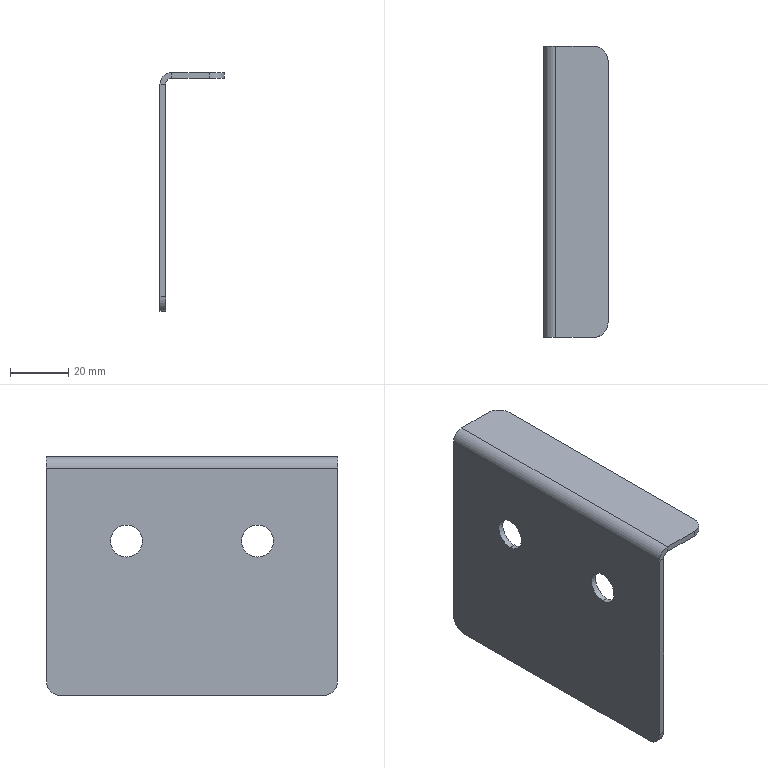Part | SolidWorks | features Fillet 1, FlatPattern 1, ICE 1, SMBaseFlange 1, SheetMetal 1 | 1 solid | 22 faces | box 22 x 100 x 82 mm | volume 19719 mm3 | plane 12 | cylinder 10 | commonest cylinder face diameters 10 x4 11 x4 4 x1 8 x1
STEP:
#1=CARTESIAN_POINT('',(0.,22.5,-32.5));
#2=VERTEX_POINT('',#1);
#3=CARTESIAN_POINT('',(0.,22.5,-21.5));
#4=VERTEX_POINT('',#3);
#5=CARTESIAN_POINT('',(0.,22.5,-27.));
#6=DIRECTION('',(-1.,0.,0.));
#7=DIRECTION('',(0.,0.,1.));
#8=AXIS2_PLACEMENT_3D('',#5,#6,#7);
#9=CIRCLE('',#8,5.5);
#10=EDGE_CURVE('',#2,#4,#9,.T.);
#11=ORIENTED_EDGE('',*,*,#10,.F.);
#12=CARTESIAN_POINT('',(-2.,22.5,-32.5));
#13=VERTEX_POINT('',#12);
#14=CARTESIAN_POINT('',(0.,22.5,-32.5));
#15=DIRECTION('',(-1.,0.,0.));
#16=VECTOR('',#15,1000.);
#17=LINE('',#14,#16);
#18=EDGE_CURVE('',#2,#13,#17,.T.);
#19=ORIENTED_EDGE('',*,*,#18,.T.);
#20=CARTESIAN_POINT('',(-2.,22.5,-21.5));
#21=VERTEX_POINT('',#20);
#22=CARTESIAN_POINT('',(-2.,22.5,-27.));
#23=DIRECTION('',(-1.,0.,0.));
#24=DIRECTION('',(0.,0.,1.));
#25=AXIS2_PLACEMENT_3D('',#22,#23,#24);
#26=CIRCLE('',#25,5.5);
#27=EDGE_CURVE('',#13,#21,#26,.T.);
#28=ORIENTED_EDGE('',*,*,#27,.T.);
#29=CARTESIAN_POINT('',(0.,22.5,-21.5));
#30=DIRECTION('',(-1.,0.,0.));
#31=VECTOR('',#30,1000.);
#32=LINE('',#29,#31);
#33=EDGE_CURVE('',#4,#21,#32,.T.);
#34=ORIENTED_EDGE('',*,*,#33,.F.);
#35=EDGE_LOOP('',(#11,#19,#28,#34));
#36=FACE_OUTER_BOUND('',#35,.T.);
#37=CARTESIAN_POINT('',(0.,22.5,-27.));
#38=DIRECTION('',(-1.,0.,0.));
#39=DIRECTION('',(0.,0.,1.));
#40=AXIS2_PLACEMENT_3D('',#37,#38,#39);
#41=CYLINDRICAL_SURFACE('',#40,5.5);
#42=ADVANCED_FACE('',(#36),#41,.F.);
#43=CARTESIAN_POINT('',(0.,-22.5,-32.5));
#44=VERTEX_POINT('',#43);
#45=CARTESIAN_POINT('',(0.,-22.5,-21.5));
#46=VERTEX_POINT('',#45);
#47=CARTESIAN_POINT('',(0.,-22.5,-27.));
#48=DIRECTION('',(-1.,0.,0.));
#49=DIRECTION('',(0.,0.,-1.));
#50=AXIS2_PLACEMENT_3D('',#47,#48,#49);
#51=CIRCLE('',#50,5.5);
#52=EDGE_CURVE('',#44,#46,#51,.T.);
#53=ORIENTED_EDGE('',*,*,#52,.F.);
#54=CARTESIAN_POINT('',(-2.,-22.5,-32.5));
#55=VERTEX_POINT('',#54);
#56=CARTESIAN_POINT('',(0.,-22.5,-32.5));
#57=DIRECTION('',(-1.,0.,0.));
#58=VECTOR('',#57,1000.);
#59=LINE('',#56,#58);
#60=EDGE_CURVE('',#44,#55,#59,.T.);
#61=ORIENTED_EDGE('',*,*,#60,.T.);
#62=CARTESIAN_POINT('',(-2.,-22.5,-21.5));
#63=VERTEX_POINT('',#62);
#64=CARTESIAN_POINT('',(-2.,-22.5,-27.));
#65=DIRECTION('',(-1.,0.,0.));
#66=DIRECTION('',(0.,0.,-1.));
#67=AXIS2_PLACEMENT_3D('',#64,#65,#66);
#68=CIRCLE('',#67,5.5);
#69=EDGE_CURVE('',#55,#63,#68,.T.);
#70=ORIENTED_EDGE('',*,*,#69,.T.);
#71=CARTESIAN_POINT('',(0.,-22.5,-21.5));
#72=DIRECTION('',(-1.,0.,0.));
#73=VECTOR('',#72,1000.);
#74=LINE('',#71,#73);
#75=EDGE_CURVE('',#46,#63,#74,.T.);
#76=ORIENTED_EDGE('',*,*,#75,.F.);
#77=EDGE_LOOP('',(#53,#61,#70,#76));
#78=FACE_OUTER_BOUND('',#77,.T.);
#79=CARTESIAN_POINT('',(0.,-22.5,-27.));
#80=DIRECTION('',(-1.,0.,0.));
#81=DIRECTION('',(0.,0.,1.));
#82=AXIS2_PLACEMENT_3D('',#79,#80,#81);
#83=CYLINDRICAL_SURFACE('',#82,5.5);
#84=ADVANCED_FACE('',(#78),#83,.F.);
#85=CARTESIAN_POINT('',(2.,50.,0.));
#86=VERTEX_POINT('',#85);
#87=CARTESIAN_POINT('',(2.,50.,2.));
#88=VERTEX_POINT('',#87);
#89=CARTESIAN_POINT('',(2.,50.,0.));
#90=DIRECTION('',(0.,0.,1.));
#91=VECTOR('',#90,1000.);
#92=LINE('',#89,#91);
#93=EDGE_CURVE('',#86,#88,#92,.T.);
#94=ORIENTED_EDGE('',*,*,#93,.F.);
#95=CARTESIAN_POINT('',(0.,50.,-2.));
#96=VERTEX_POINT('',#95);
#97=CARTESIAN_POINT('',(2.,50.,-2.));
#98=DIRECTION('',(0.,1.,0.));
#99=DIRECTION('',(0.,0.,-1.));
#100=AXIS2_PLACEMENT_3D('',#97,#98,#99);
#101=CIRCLE('',#100,2.);
#102=EDGE_CURVE('',#96,#86,#101,.T.);
#103=ORIENTED_EDGE('',*,*,#102,.F.);
#104=CARTESIAN_POINT('',(-2.,50.,-2.));
#105=VERTEX_POINT('',#104);
#106=CARTESIAN_POINT('',(-2.,50.,-2.));
#107=DIRECTION('',(1.,0.,0.));
#108=VECTOR('',#107,1000.);
#109=LINE('',#106,#108);
#110=EDGE_CURVE('',#105,#96,#109,.T.);
#111=ORIENTED_EDGE('',*,*,#110,.F.);
#112=CARTESIAN_POINT('',(2.,50.,-2.));
#113=DIRECTION('',(0.,1.,0.));
#114=DIRECTION('',(1.,0.,0.));
#115=AXIS2_PLACEMENT_3D('',#112,#113,#114);
#116=CIRCLE('',#115,4.);
#117=EDGE_CURVE('',#105,#88,#116,.T.);
#118=ORIENTED_EDGE('',*,*,#117,.T.);
#119=EDGE_LOOP('',(#94,#103,#111,#118));
#120=FACE_OUTER_BOUND('',#119,.T.);
#121=CARTESIAN_POINT('',(2.,50.,0.));
#122=DIRECTION('',(0.,1.,0.));
#123=DIRECTION('',(0.,0.,1.));
#124=AXIS2_PLACEMENT_3D('',#121,#122,#123);
#125=PLANE('',#124);
#126=ADVANCED_FACE('',(#120),#125,.T.);
#127=CARTESIAN_POINT('',(15.,50.,2.));
#128=VERTEX_POINT('',#127);
#129=CARTESIAN_POINT('',(0.,50.,2.));
#130=DIRECTION('',(1.,0.,0.));
#131=VECTOR('',#130,1000.);
#132=LINE('',#129,#131);
#133=EDGE_CURVE('',#88,#128,#132,.T.);
#134=ORIENTED_EDGE('',*,*,#133,.T.);
#135=CARTESIAN_POINT('',(15.,50.,0.));
#136=VERTEX_POINT('',#135);
#137=CARTESIAN_POINT('',(15.,50.,-2.));
#138=DIRECTION('',(0.,0.,-1.));
#139=VECTOR('',#138,1000.);
#140=LINE('',#137,#139);
#141=EDGE_CURVE('',#128,#136,#140,.T.);
#142=ORIENTED_EDGE('',*,*,#141,.T.);
#143=CARTESIAN_POINT('',(0.,50.,0.));
#144=DIRECTION('',(1.,0.,0.));
#145=VECTOR('',#144,1000.);
#146=LINE('',#143,#145);
#147=EDGE_CURVE('',#86,#136,#146,.T.);
#148=ORIENTED_EDGE('',*,*,#147,.F.);
#149=ORIENTED_EDGE('',*,*,#93,.T.);
#150=EDGE_LOOP('',(#134,#142,#148,#149));
#151=FACE_OUTER_BOUND('',#150,.T.);
#152=CARTESIAN_POINT('',(-2.,50.,-2.));
#153=DIRECTION('',(0.,1.,0.));
#154=DIRECTION('',(0.,0.,1.));
#155=AXIS2_PLACEMENT_3D('',#152,#153,#154);
#156=PLANE('',#155);
#157=ADVANCED_FACE('',(#151),#156,.T.);
#158=CARTESIAN_POINT('',(0.,-50.,-2.));
#159=VERTEX_POINT('',#158);
#160=CARTESIAN_POINT('',(-2.,-50.,-2.));
#161=VERTEX_POINT('',#160);
#162=CARTESIAN_POINT('',(0.,-50.,-2.));
#163=DIRECTION('',(-1.,0.,0.));
#164=VECTOR('',#163,1000.);
#165=LINE('',#162,#164);
#166=EDGE_CURVE('',#159,#161,#165,.T.);
#167=ORIENTED_EDGE('',*,*,#166,.F.);
#168=CARTESIAN_POINT('',(2.,-50.,0.));
#169=VERTEX_POINT('',#168);
#170=CARTESIAN_POINT('',(2.,-50.,-2.));
#171=DIRECTION('',(0.,1.,0.));
#172=DIRECTION('',(0.,0.,-1.));
#173=AXIS2_PLACEMENT_3D('',#170,#171,#172);
#174=CIRCLE('',#173,2.);
#175=EDGE_CURVE('',#159,#169,#174,.T.);
#176=ORIENTED_EDGE('',*,*,#175,.T.);
#177=CARTESIAN_POINT('',(2.,-50.,2.));
#178=VERTEX_POINT('',#177);
#179=CARTESIAN_POINT('',(2.,-50.,2.));
#180=DIRECTION('',(0.,0.,-1.));
#181=VECTOR('',#180,1000.);
#182=LINE('',#179,#181);
#183=EDGE_CURVE('',#178,#169,#182,.T.);
#184=ORIENTED_EDGE('',*,*,#183,.F.);
#185=CARTESIAN_POINT('',(2.,-50.,-2.));
#186=DIRECTION('',(0.,1.,0.));
#187=DIRECTION('',(1.,0.,0.));
#188=AXIS2_PLACEMENT_3D('',#185,#186,#187);
#189=CIRCLE('',#188,4.);
#190=EDGE_CURVE('',#161,#178,#189,.T.);
#191=ORIENTED_EDGE('',*,*,#190,.F.);
#192=EDGE_LOOP('',(#167,#176,#184,#191));
#193=FACE_OUTER_BOUND('',#192,.T.);
#194=CARTESIAN_POINT('',(0.,-50.,-2.));
#195=DIRECTION('',(0.,-1.,0.));
#196=DIRECTION('',(0.,0.,-1.));
#197=AXIS2_PLACEMENT_3D('',#194,#195,#196);
#198=PLANE('',#197);
#199=ADVANCED_FACE('',(#193),#198,.T.);
#200=CARTESIAN_POINT('',(-2.,-50.,-75.));
#201=VERTEX_POINT('',#200);
#202=CARTESIAN_POINT('',(-2.,-50.,-80.));
#203=DIRECTION('',(0.,0.,1.));
#204=VECTOR('',#203,1000.);
#205=LINE('',#202,#204);
#206=EDGE_CURVE('',#201,#161,#205,.T.);
#207=ORIENTED_EDGE('',*,*,#206,.F.);
#208=CARTESIAN_POINT('',(0.,-50.,-75.));
#209=VERTEX_POINT('',#208);
#210=CARTESIAN_POINT('',(2.,-50.,-75.));
#211=DIRECTION('',(1.,0.,0.));
#212=VECTOR('',#211,1000.);
#213=LINE('',#210,#212);
#214=EDGE_CURVE('',#201,#209,#213,.T.);
#215=ORIENTED_EDGE('',*,*,#214,.T.);
#216=CARTESIAN_POINT('',(0.,-50.,-80.));
#217=DIRECTION('',(0.,0.,1.));
#218=VECTOR('',#217,1000.);
#219=LINE('',#216,#218);
#220=EDGE_CURVE('',#209,#159,#219,.T.);
#221=ORIENTED_EDGE('',*,*,#220,.T.);
#222=ORIENTED_EDGE('',*,*,#166,.T.);
#223=EDGE_LOOP('',(#207,#215,#221,#222));
#224=FACE_OUTER_BOUND('',#223,.T.);
#225=CARTESIAN_POINT('',(2.,-50.,2.));
#226=DIRECTION('',(0.,-1.,0.));
#227=DIRECTION('',(0.,0.,-1.));
#228=AXIS2_PLACEMENT_3D('',#225,#226,#227);
#229=PLANE('',#228);
#230=ADVANCED_FACE('',(#224),#229,.T.);
#231=CARTESIAN_POINT('',(20.,45.,2.));
#232=VERTEX_POINT('',#231);
#233=CARTESIAN_POINT('',(20.,-45.,2.));
#234=VERTEX_POINT('',#233);
#235=CARTESIAN_POINT('',(20.,50.,2.));
#236=DIRECTION('',(0.,-1.,0.));
#237=VECTOR('',#236,1000.);
#238=LINE('',#235,#237);
#239=EDGE_CURVE('',#232,#234,#238,.T.);
#240=ORIENTED_EDGE('',*,*,#239,.F.);
#241=CARTESIAN_POINT('',(15.,45.,2.));
#242=DIRECTION('',(0.,0.,1.));
#243=DIRECTION('',(-1.,0.,0.));
#244=AXIS2_PLACEMENT_3D('',#241,#242,#243);
#245=CIRCLE('',#244,5.);
#246=EDGE_CURVE('',#232,#128,#245,.T.);
#247=ORIENTED_EDGE('',*,*,#246,.T.);
#248=ORIENTED_EDGE('',*,*,#133,.F.);
#249=CARTESIAN_POINT('',(2.,50.,2.));
#250=DIRECTION('',(0.,-1.,0.));
#251=VECTOR('',#250,1000.);
#252=LINE('',#249,#251);
#253=EDGE_CURVE('',#88,#178,#252,.T.);
#254=ORIENTED_EDGE('',*,*,#253,.T.);
#255=CARTESIAN_POINT('',(15.,-50.,2.));
#256=VERTEX_POINT('',#255);
#257=CARTESIAN_POINT('',(0.,-50.,2.));
#258=DIRECTION('',(1.,0.,0.));
#259=VECTOR('',#258,1000.);
#260=LINE('',#257,#259);
#261=EDGE_CURVE('',#178,#256,#260,.T.);
#262=ORIENTED_EDGE('',*,*,#261,.T.);
#263=CARTESIAN_POINT('',(15.,-45.,2.));
#264=DIRECTION('',(0.,0.,1.));
#265=DIRECTION('',(-1.,0.,0.));
#266=AXIS2_PLACEMENT_3D('',#263,#264,#265);
#267=CIRCLE('',#266,5.);
#268=EDGE_CURVE('',#256,#234,#267,.T.);
#269=ORIENTED_EDGE('',*,*,#268,.T.);
#270=EDGE_LOOP('',(#240,#247,#248,#254,#262,#269));
#271=FACE_OUTER_BOUND('',#270,.T.);
#272=CARTESIAN_POINT('',(0.,50.,2.));
#273=DIRECTION('',(0.,0.,-1.));
#274=DIRECTION('',(-1.,0.,0.));
#275=AXIS2_PLACEMENT_3D('',#272,#273,#274);
#276=PLANE('',#275);
#277=ADVANCED_FACE('',(#271),#276,.F.);
#278=CARTESIAN_POINT('',(20.,45.,0.));
#279=VERTEX_POINT('',#278);
#280=CARTESIAN_POINT('',(20.,-45.,0.));
#281=VERTEX_POINT('',#280);
#282=CARTESIAN_POINT('',(20.,50.,0.));
#283=DIRECTION('',(0.,-1.,0.));
#284=VECTOR('',#283,1000.);
#285=LINE('',#282,#284);
#286=EDGE_CURVE('',#279,#281,#285,.T.);
#287=ORIENTED_EDGE('',*,*,#286,.F.);
#288=CARTESIAN_POINT('',(20.,45.,0.));
#289=DIRECTION('',(0.,0.,1.));
#290=VECTOR('',#289,1000.);
#291=LINE('',#288,#290);
#292=EDGE_CURVE('',#279,#232,#291,.T.);
#293=ORIENTED_EDGE('',*,*,#292,.T.);
#294=ORIENTED_EDGE('',*,*,#239,.T.);
#295=CARTESIAN_POINT('',(20.,-45.,0.));
#296=DIRECTION('',(0.,0.,-1.));
#297=VECTOR('',#296,1000.);
#298=LINE('',#295,#297);
#299=EDGE_CURVE('',#234,#281,#298,.T.);
#300=ORIENTED_EDGE('',*,*,#299,.T.);
#301=EDGE_LOOP('',(#287,#293,#294,#300));
#302=FACE_OUTER_BOUND('',#301,.T.);
#303=CARTESIAN_POINT('',(20.,50.,0.));
#304=DIRECTION('',(1.,0.,0.));
#305=DIRECTION('',(0.,0.,-1.));
#306=AXIS2_PLACEMENT_3D('',#303,#304,#305);
#307=PLANE('',#306);
#308=ADVANCED_FACE('',(#302),#307,.T.);
#309=ORIENTED_EDGE('',*,*,#147,.T.);
#310=CARTESIAN_POINT('',(15.,45.,0.));
#311=DIRECTION('',(0.,0.,-1.));
#312=DIRECTION('',(-1.,0.,0.));
#313=AXIS2_PLACEMENT_3D('',#310,#311,#312);
#314=CIRCLE('',#313,5.);
#315=EDGE_CURVE('',#136,#279,#314,.T.);
#316=ORIENTED_EDGE('',*,*,#315,.T.);
#317=ORIENTED_EDGE('',*,*,#286,.T.);
#318=CARTESIAN_POINT('',(15.,-50.,0.));
#319=VERTEX_POINT('',#318);
#320=CARTESIAN_POINT('',(15.,-45.,0.));
#321=DIRECTION('',(0.,0.,-1.));
#322=DIRECTION('',(-1.,0.,0.));
#323=AXIS2_PLACEMENT_3D('',#320,#321,#322);
#324=CIRCLE('',#323,5.);
#325=EDGE_CURVE('',#281,#319,#324,.T.);
#326=ORIENTED_EDGE('',*,*,#325,.T.);
#327=CARTESIAN_POINT('',(0.,-50.,0.));
#328=DIRECTION('',(1.,0.,0.));
#329=VECTOR('',#328,1000.);
#330=LINE('',#327,#329);
#331=EDGE_CURVE('',#169,#319,#330,.T.);
#332=ORIENTED_EDGE('',*,*,#331,.F.);
#333=CARTESIAN_POINT('',(2.,50.,0.));
#334=DIRECTION('',(0.,-1.,0.));
#335=VECTOR('',#334,1000.);
#336=LINE('',#333,#335);
#337=EDGE_CURVE('',#86,#169,#336,.T.);
#338=ORIENTED_EDGE('',*,*,#337,.F.);
#339=EDGE_LOOP('',(#309,#316,#317,#326,#332,#338));
#340=FACE_OUTER_BOUND('',#339,.T.);
#341=CARTESIAN_POINT('',(0.,50.,0.));
#342=DIRECTION('',(0.,0.,-1.));
#343=DIRECTION('',(-1.,0.,0.));
#344=AXIS2_PLACEMENT_3D('',#341,#342,#343);
#345=PLANE('',#344);
#346=ADVANCED_FACE('',(#340),#345,.T.);
#347=ORIENTED_EDGE('',*,*,#175,.F.);
#348=CARTESIAN_POINT('',(0.,50.,-2.));
#349=DIRECTION('',(0.,-1.,0.));
#350=VECTOR('',#349,1000.);
#351=LINE('',#348,#350);
#352=EDGE_CURVE('',#96,#159,#351,.T.);
#353=ORIENTED_EDGE('',*,*,#352,.F.);
#354=ORIENTED_EDGE('',*,*,#102,.T.);
#355=ORIENTED_EDGE('',*,*,#337,.T.);
#356=EDGE_LOOP('',(#347,#353,#354,#355));
#357=FACE_OUTER_BOUND('',#356,.T.);
#358=CARTESIAN_POINT('',(2.,50.,-2.));
#359=DIRECTION('',(0.,-1.,0.));
#360=DIRECTION('',(0.,0.,-1.));
#361=AXIS2_PLACEMENT_3D('',#358,#359,#360);
#362=CYLINDRICAL_SURFACE('',#361,2.);
#363=ADVANCED_FACE('',(#357),#362,.F.);
#364=CARTESIAN_POINT('',(0.,22.5,-27.));
#365=DIRECTION('',(-1.,0.,0.));
#366=DIRECTION('',(0.,0.,1.));
#367=AXIS2_PLACEMENT_3D('',#364,#365,#366);
#368=CIRCLE('',#367,5.5);
#369=EDGE_CURVE('',#4,#2,#368,.T.);
#370=ORIENTED_EDGE('',*,*,#369,.T.);
#371=ORIENTED_EDGE('',*,*,#10,.T.);
#372=EDGE_LOOP('',(#370,#371));
#373=FACE_BOUND('',#372,.T.);
#374=CARTESIAN_POINT('',(0.,-22.5,-27.));
#375=DIRECTION('',(-1.,0.,0.));
#376=DIRECTION('',(0.,0.,-1.));
#377=AXIS2_PLACEMENT_3D('',#374,#375,#376);
#378=CIRCLE('',#377,5.5);
#379=EDGE_CURVE('',#46,#44,#378,.T.);
#380=ORIENTED_EDGE('',*,*,#379,.T.);
#381=ORIENTED_EDGE('',*,*,#52,.T.);
#382=EDGE_LOOP('',(#380,#381));
#383=FACE_BOUND('',#382,.T.);
#384=ORIENTED_EDGE('',*,*,#220,.F.);
#385=CARTESIAN_POINT('',(0.,-45.,-80.));
#386=VERTEX_POINT('',#385);
#387=CARTESIAN_POINT('',(0.,-45.,-75.));
#388=DIRECTION('',(1.,0.,0.));
#389=DIRECTION('',(0.,0.,-1.));
#390=AXIS2_PLACEMENT_3D('',#387,#388,#389);
#391=CIRCLE('',#390,5.);
#392=EDGE_CURVE('',#209,#386,#391,.T.);
#393=ORIENTED_EDGE('',*,*,#392,.T.);
#394=CARTESIAN_POINT('',(0.,45.,-80.));
#395=VERTEX_POINT('',#394);
#396=CARTESIAN_POINT('',(0.,50.,-80.));
#397=DIRECTION('',(0.,-1.,0.));
#398=VECTOR('',#397,1000.);
#399=LINE('',#396,#398);
#400=EDGE_CURVE('',#395,#386,#399,.T.);
#401=ORIENTED_EDGE('',*,*,#400,.F.);
#402=CARTESIAN_POINT('',(0.,50.,-75.));
#403=VERTEX_POINT('',#402);
#404=CARTESIAN_POINT('',(0.,45.,-75.));
#405=DIRECTION('',(1.,0.,0.));
#406=DIRECTION('',(0.,0.,-1.));
#407=AXIS2_PLACEMENT_3D('',#404,#405,#406);
#408=CIRCLE('',#407,5.);
#409=EDGE_CURVE('',#395,#403,#408,.T.);
#410=ORIENTED_EDGE('',*,*,#409,.T.);
#411=CARTESIAN_POINT('',(0.,50.,-80.));
#412=DIRECTION('',(0.,0.,1.));
#413=VECTOR('',#412,1000.);
#414=LINE('',#411,#413);
#415=EDGE_CURVE('',#403,#96,#414,.T.);
#416=ORIENTED_EDGE('',*,*,#415,.T.);
#417=ORIENTED_EDGE('',*,*,#352,.T.);
#418=EDGE_LOOP('',(#384,#393,#401,#410,#416,#417));
#419=FACE_OUTER_BOUND('',#418,.T.);
#420=CARTESIAN_POINT('',(0.,50.,-80.));
#421=DIRECTION('',(1.,0.,0.));
#422=DIRECTION('',(0.,0.,-1.));
#423=AXIS2_PLACEMENT_3D('',#420,#421,#422);
#424=PLANE('',#423);
#425=ADVANCED_FACE('',(#373,#383,#419),#424,.T.);
#426=ORIENTED_EDGE('',*,*,#400,.T.);
#427=CARTESIAN_POINT('',(-2.,-45.,-80.));
#428=VERTEX_POINT('',#427);
#429=CARTESIAN_POINT('',(-2.,-45.,-80.));
#430=DIRECTION('',(-1.,0.,0.));
#431=VECTOR('',#430,1000.);
#432=LINE('',#429,#431);
#433=EDGE_CURVE('',#386,#428,#432,.T.);
#434=ORIENTED_EDGE('',*,*,#433,.T.);
#435=CARTESIAN_POINT('',(-2.,45.,-80.));
#436=VERTEX_POINT('',#435);
#437=CARTESIAN_POINT('',(-2.,50.,-80.));
#438=DIRECTION('',(0.,-1.,0.));
#439=VECTOR('',#438,1000.);
#440=LINE('',#437,#439);
#441=EDGE_CURVE('',#436,#428,#440,.T.);
#442=ORIENTED_EDGE('',*,*,#441,.F.);
#443=CARTESIAN_POINT('',(0.,45.,-80.));
#444=DIRECTION('',(1.,0.,0.));
#445=VECTOR('',#444,1000.);
#446=LINE('',#443,#445);
#447=EDGE_CURVE('',#436,#395,#446,.T.);
#448=ORIENTED_EDGE('',*,*,#447,.T.);
#449=EDGE_LOOP('',(#426,#434,#442,#448));
#450=FACE_OUTER_BOUND('',#449,.T.);
#451=CARTESIAN_POINT('',(-2.,50.,-80.));
#452=DIRECTION('',(0.,0.,-1.));
#453=DIRECTION('',(-1.,0.,0.));
#454=AXIS2_PLACEMENT_3D('',#451,#452,#453);
#455=PLANE('',#454);
#456=ADVANCED_FACE('',(#450),#455,.T.);
#457=CARTESIAN_POINT('',(-2.,22.5,-27.));
#458=DIRECTION('',(-1.,0.,0.));
#459=DIRECTION('',(0.,0.,1.));
#460=AXIS2_PLACEMENT_3D('',#457,#458,#459);
#461=CIRCLE('',#460,5.5);
#462=EDGE_CURVE('',#21,#13,#461,.T.);
#463=ORIENTED_EDGE('',*,*,#462,.F.);
#464=ORIENTED_EDGE('',*,*,#27,.F.);
#465=EDGE_LOOP('',(#463,#464));
#466=FACE_BOUND('',#465,.T.);
#467=CARTESIAN_POINT('',(-2.,-22.5,-27.));
#468=DIRECTION('',(-1.,0.,0.));
#469=DIRECTION('',(0.,0.,-1.));
#470=AXIS2_PLACEMENT_3D('',#467,#468,#469);
#471=CIRCLE('',#470,5.5);
#472=EDGE_CURVE('',#63,#55,#471,.T.);
#473=ORIENTED_EDGE('',*,*,#472,.F.);
#474=ORIENTED_EDGE('',*,*,#69,.F.);
#475=EDGE_LOOP('',(#473,#474));
#476=FACE_BOUND('',#475,.T.);
#477=ORIENTED_EDGE('',*,*,#441,.T.);
#478=CARTESIAN_POINT('',(-2.,-45.,-75.));
#479=DIRECTION('',(-1.,0.,0.));
#480=DIRECTION('',(0.,0.,-1.));
#481=AXIS2_PLACEMENT_3D('',#478,#479,#480);
#482=CIRCLE('',#481,5.);
#483=EDGE_CURVE('',#428,#201,#482,.T.);
#484=ORIENTED_EDGE('',*,*,#483,.T.);
#485=ORIENTED_EDGE('',*,*,#206,.T.);
#486=CARTESIAN_POINT('',(-2.,50.,-2.));
#487=DIRECTION('',(0.,-1.,0.));
#488=VECTOR('',#487,1000.);
#489=LINE('',#486,#488);
#490=EDGE_CURVE('',#105,#161,#489,.T.);
#491=ORIENTED_EDGE('',*,*,#490,.F.);
#492=CARTESIAN_POINT('',(-2.,50.,-75.));
#493=VERTEX_POINT('',#492);
#494=CARTESIAN_POINT('',(-2.,50.,-80.));
#495=DIRECTION('',(0.,0.,1.));
#496=VECTOR('',#495,1000.);
#497=LINE('',#494,#496);
#498=EDGE_CURVE('',#493,#105,#497,.T.);
#499=ORIENTED_EDGE('',*,*,#498,.F.);
#500=CARTESIAN_POINT('',(-2.,45.,-75.));
#501=DIRECTION('',(-1.,0.,0.));
#502=DIRECTION('',(0.,0.,-1.));
#503=AXIS2_PLACEMENT_3D('',#500,#501,#502);
#504=CIRCLE('',#503,5.);
#505=EDGE_CURVE('',#493,#436,#504,.T.);
#506=ORIENTED_EDGE('',*,*,#505,.T.);
#507=EDGE_LOOP('',(#477,#484,#485,#491,#499,#506));
#508=FACE_OUTER_BOUND('',#507,.T.);
#509=CARTESIAN_POINT('',(-2.,50.,-80.));
#510=DIRECTION('',(1.,0.,0.));
#511=DIRECTION('',(0.,0.,-1.));
#512=AXIS2_PLACEMENT_3D('',#509,#510,#511);
#513=PLANE('',#512);
#514=ADVANCED_FACE('',(#466,#476,#508),#513,.F.);
#515=ORIENTED_EDGE('',*,*,#190,.T.);
#516=ORIENTED_EDGE('',*,*,#253,.F.);
#517=ORIENTED_EDGE('',*,*,#117,.F.);
#518=ORIENTED_EDGE('',*,*,#490,.T.);
#519=EDGE_LOOP('',(#515,#516,#517,#518));
#520=FACE_OUTER_BOUND('',#519,.T.);
#521=CARTESIAN_POINT('',(2.,50.,-2.));
#522=DIRECTION('',(0.,-1.,0.));
#523=DIRECTION('',(0.,0.,-1.));
#524=AXIS2_PLACEMENT_3D('',#521,#522,#523);
#525=CYLINDRICAL_SURFACE('',#524,4.);
#526=ADVANCED_FACE('',(#520),#525,.T.);
#527=ORIENTED_EDGE('',*,*,#415,.F.);
#528=CARTESIAN_POINT('',(-2.,50.,-75.));
#529=DIRECTION('',(-1.,0.,0.));
#530=VECTOR('',#529,1000.);
#531=LINE('',#528,#530);
#532=EDGE_CURVE('',#403,#493,#531,.T.);
#533=ORIENTED_EDGE('',*,*,#532,.T.);
#534=ORIENTED_EDGE('',*,*,#498,.T.);
#535=ORIENTED_EDGE('',*,*,#110,.T.);
#536=EDGE_LOOP('',(#527,#533,#534,#535));
#537=FACE_OUTER_BOUND('',#536,.T.);
#538=CARTESIAN_POINT('',(2.,50.,-2.));
#539=DIRECTION('',(0.,-1.,0.));
#540=DIRECTION('',(-1.,0.,0.));
#541=AXIS2_PLACEMENT_3D('',#538,#539,#540);
#542=PLANE('',#541);
#543=ADVANCED_FACE('',(#537),#542,.F.);
#544=ORIENTED_EDGE('',*,*,#331,.T.);
#545=CARTESIAN_POINT('',(15.,-50.,-2.));
#546=DIRECTION('',(0.,0.,1.));
#547=VECTOR('',#546,1000.);
#548=LINE('',#545,#547);
#549=EDGE_CURVE('',#319,#256,#548,.T.);
#550=ORIENTED_EDGE('',*,*,#549,.T.);
#551=ORIENTED_EDGE('',*,*,#261,.F.);
#552=ORIENTED_EDGE('',*,*,#183,.T.);
#553=EDGE_LOOP('',(#544,#550,#551,#552));
#554=FACE_OUTER_BOUND('',#553,.T.);
#555=CARTESIAN_POINT('',(2.,-50.,-2.));
#556=DIRECTION('',(0.,-1.,0.));
#557=DIRECTION('',(-1.,0.,0.));
#558=AXIS2_PLACEMENT_3D('',#555,#556,#557);
#559=PLANE('',#558);
#560=ADVANCED_FACE('',(#554),#559,.T.);
#561=ORIENTED_EDGE('',*,*,#60,.F.);
#562=ORIENTED_EDGE('',*,*,#379,.F.);
#563=ORIENTED_EDGE('',*,*,#75,.T.);
#564=ORIENTED_EDGE('',*,*,#472,.T.);
#565=EDGE_LOOP('',(#561,#562,#563,#564));
#566=FACE_OUTER_BOUND('',#565,.T.);
#567=CARTESIAN_POINT('',(0.,-22.5,-27.));
#568=DIRECTION('',(-1.,0.,0.));
#569=DIRECTION('',(0.,0.,1.));
#570=AXIS2_PLACEMENT_3D('',#567,#568,#569);
#571=CYLINDRICAL_SURFACE('',#570,5.5);
#572=ADVANCED_FACE('',(#566),#571,.F.);
#573=ORIENTED_EDGE('',*,*,#18,.F.);
#574=ORIENTED_EDGE('',*,*,#369,.F.);
#575=ORIENTED_EDGE('',*,*,#33,.T.);
#576=ORIENTED_EDGE('',*,*,#462,.T.);
#577=EDGE_LOOP('',(#573,#574,#575,#576));
#578=FACE_OUTER_BOUND('',#577,.T.);
#579=CARTESIAN_POINT('',(0.,22.5,-27.));
#580=DIRECTION('',(-1.,0.,0.));
#581=DIRECTION('',(0.,0.,1.));
#582=AXIS2_PLACEMENT_3D('',#579,#580,#581);
#583=CYLINDRICAL_SURFACE('',#582,5.5);
#584=ADVANCED_FACE('',(#578),#583,.F.);
#585=ORIENTED_EDGE('',*,*,#315,.F.);
#586=ORIENTED_EDGE('',*,*,#141,.F.);
#587=ORIENTED_EDGE('',*,*,#246,.F.);
#588=ORIENTED_EDGE('',*,*,#292,.F.);
#589=EDGE_LOOP('',(#585,#586,#587,#588));
#590=FACE_OUTER_BOUND('',#589,.T.);
#591=CARTESIAN_POINT('',(15.,45.,0.));
#592=DIRECTION('',(0.,0.,1.));
#593=DIRECTION('',(1.,0.,0.));
#594=AXIS2_PLACEMENT_3D('',#591,#592,#593);
#595=CYLINDRICAL_SURFACE('',#594,5.);
#596=ADVANCED_FACE('',(#590),#595,.T.);
#597=ORIENTED_EDGE('',*,*,#325,.F.);
#598=ORIENTED_EDGE('',*,*,#299,.F.);
#599=ORIENTED_EDGE('',*,*,#268,.F.);
#600=ORIENTED_EDGE('',*,*,#549,.F.);
#601=EDGE_LOOP('',(#597,#598,#599,#600));
#602=FACE_OUTER_BOUND('',#601,.T.);
#603=CARTESIAN_POINT('',(15.,-45.,-2.));
#604=DIRECTION('',(0.,0.,1.));
#605=DIRECTION('',(1.,0.,0.));
#606=AXIS2_PLACEMENT_3D('',#603,#604,#605);
#607=CYLINDRICAL_SURFACE('',#606,5.);
#608=ADVANCED_FACE('',(#602),#607,.T.);
#609=ORIENTED_EDGE('',*,*,#483,.F.);
#610=ORIENTED_EDGE('',*,*,#433,.F.);
#611=ORIENTED_EDGE('',*,*,#392,.F.);
#612=ORIENTED_EDGE('',*,*,#214,.F.);
#613=EDGE_LOOP('',(#609,#610,#611,#612));
#614=FACE_OUTER_BOUND('',#613,.T.);
#615=CARTESIAN_POINT('',(2.,-45.,-75.));
#616=DIRECTION('',(1.,0.,0.));
#617=DIRECTION('',(0.,0.,-1.));
#618=AXIS2_PLACEMENT_3D('',#615,#616,#617);
#619=CYLINDRICAL_SURFACE('',#618,5.);
#620=ADVANCED_FACE('',(#614),#619,.T.);
#621=ORIENTED_EDGE('',*,*,#505,.F.);
#622=ORIENTED_EDGE('',*,*,#532,.F.);
#623=ORIENTED_EDGE('',*,*,#409,.F.);
#624=ORIENTED_EDGE('',*,*,#447,.F.);
#625=EDGE_LOOP('',(#621,#622,#623,#624));
#626=FACE_OUTER_BOUND('',#625,.T.);
#627=CARTESIAN_POINT('',(-2.,45.,-75.));
#628=DIRECTION('',(-1.,0.,0.));
#629=DIRECTION('',(0.,0.,1.));
#630=AXIS2_PLACEMENT_3D('',#627,#628,#629);
#631=CYLINDRICAL_SURFACE('',#630,5.);
#632=ADVANCED_FACE('',(#626),#631,.T.);
#633=CLOSED_SHELL('',(#42,#84,#126,#157,#199,#230,#277,#308,#346,#363,#425,#456,#514,#526,#543,#560,#572,#584,#596,#608,#620,#632));
#634=MANIFOLD_SOLID_BREP('',#633);
#635=CARTESIAN_POINT('',(0.,0.,0.));
#636=DIRECTION('',(0.,0.,1.));
#637=DIRECTION('',(1.,0.,0.));
#638=AXIS2_PLACEMENT_3D('',#635,#636,#637);
#639=(LENGTH_UNIT()NAMED_UNIT(*)SI_UNIT(.MILLI.,.METRE.));
#640=UNCERTAINTY_MEASURE_WITH_UNIT(LENGTH_MEASURE(0.00001),#639,'','');
#641=(NAMED_UNIT(*)PLANE_ANGLE_UNIT()SI_UNIT($,.RADIAN.));
#642=(NAMED_UNIT(*)SI_UNIT($,.STERADIAN.)SOLID_ANGLE_UNIT());
#643=(GEOMETRIC_REPRESENTATION_CONTEXT(3)GLOBAL_UNCERTAINTY_ASSIGNED_CONTEXT((#640))GLOBAL_UNIT_ASSIGNED_CONTEXT((#639,#641,#642))REPRESENTATION_CONTEXT('',''));
#644=ADVANCED_BREP_SHAPE_REPRESENTATION('',(#634,#638),#643);